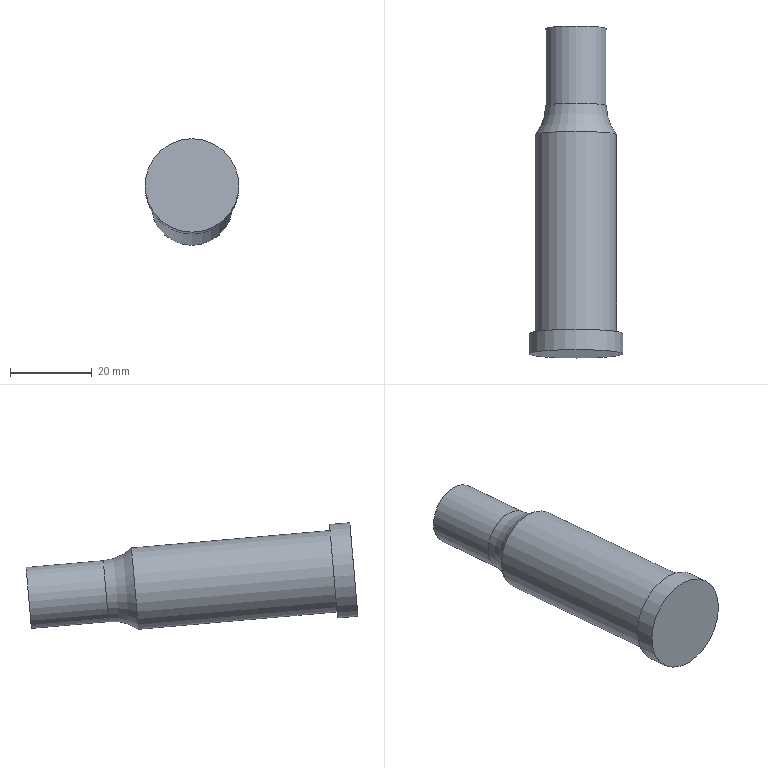Part | NX | features SPAS 20-80-18.00 2 | 1 solid | 7 faces | box 23 x 81.352 x 26.111 mm | volume 22338 mm3 | plane 3 | cylinder 3 | torus 1 | commonest cylinder face diameters 15 x1 20 x1 23 x1
STEP:
#1=CARTESIAN_POINT('',(-462.881,-59.853,-32.241));
#2=VERTEX_POINT('',#1);
#3=CARTESIAN_POINT('',(-462.881,-60.507,-39.712));
#4=DIRECTION('',(0.,0.9962,-0.08716));
#5=DIRECTION('',(0.,0.08716,0.9962));
#6=AXIS2_PLACEMENT_3D('',#3,#4,#5);
#7=CIRCLE('',#6,7.5);
#8=EDGE_CURVE('',#2,#2,#7,.F.);
#9=ORIENTED_EDGE('',*,*,#8,.F.);
#10=EDGE_LOOP('',(#9));
#11=FACE_BOUND('',#10,.T.);
#12=CARTESIAN_POINT('',(-462.881,-60.507,-39.712));
#13=DIRECTION('',(0.,0.9962,-0.08716));
#14=DIRECTION('',(0.,0.08716,0.9962));
#15=AXIS2_PLACEMENT_3D('',#12,#13,#14);
#16=PLANE('',#15);
#17=ADVANCED_FACE('',(#11),#16,.T.);
#18=CARTESIAN_POINT('',(-462.881,-80.088,-45.528));
#19=VERTEX_POINT('',#18);
#20=CARTESIAN_POINT('',(-462.881,-79.435,-38.056));
#21=DIRECTION('',(0.,-0.9962,0.08716));
#22=DIRECTION('',(0.,-0.08716,-0.9962));
#23=AXIS2_PLACEMENT_3D('',#20,#21,#22);
#24=CIRCLE('',#23,7.5);
#25=EDGE_CURVE('',#19,#19,#24,.F.);
#26=ORIENTED_EDGE('',*,*,#25,.T.);
#27=EDGE_LOOP('',(#26));
#28=FACE_BOUND('',#27,.T.);
#29=ORIENTED_EDGE('',*,*,#8,.T.);
#30=EDGE_LOOP('',(#29));
#31=FACE_BOUND('',#30,.T.);
#32=CARTESIAN_POINT('',(-462.881,-60.507,-39.712));
#33=DIRECTION('',(0.,-0.9962,0.08716));
#34=DIRECTION('',(0.,-0.08716,-0.9962));
#35=AXIS2_PLACEMENT_3D('',#32,#33,#34);
#36=CYLINDRICAL_SURFACE('',#35,7.5);
#37=ADVANCED_FACE('',(#28,#31),#36,.T.);
#38=CARTESIAN_POINT('',(-462.881,-134.35,-23.214));
#39=VERTEX_POINT('',#38);
#40=CARTESIAN_POINT('',(-462.881,-135.221,-33.175));
#41=DIRECTION('',(0.,0.9962,-0.08716));
#42=DIRECTION('',(0.,0.08716,0.9962));
#43=AXIS2_PLACEMENT_3D('',#40,#41,#42);
#44=CIRCLE('',#43,10.);
#45=EDGE_CURVE('',#39,#39,#44,.F.);
#46=ORIENTED_EDGE('',*,*,#45,.F.);
#47=EDGE_LOOP('',(#46));
#48=FACE_BOUND('',#47,.T.);
#49=CARTESIAN_POINT('',(-462.881,-85.695,-27.47));
#50=VERTEX_POINT('',#49);
#51=CARTESIAN_POINT('',(-462.881,-86.566,-37.432));
#52=DIRECTION('',(0.,0.9962,-0.08716));
#53=DIRECTION('',(0.,0.08716,0.9962));
#54=AXIS2_PLACEMENT_3D('',#51,#52,#53);
#55=CIRCLE('',#54,10.);
#56=EDGE_CURVE('',#50,#50,#55,.F.);
#57=ORIENTED_EDGE('',*,*,#56,.T.);
#58=EDGE_LOOP('',(#57));
#59=FACE_BOUND('',#58,.T.);
#60=CARTESIAN_POINT('',(-462.881,-83.777,-37.676));
#61=DIRECTION('',(0.,-0.9962,0.08716));
#62=DIRECTION('',(0.,-0.08716,-0.9962));
#63=AXIS2_PLACEMENT_3D('',#60,#61,#62);
#64=CYLINDRICAL_SURFACE('',#63,10.);
#65=ADVANCED_FACE('',(#48,#59),#64,.T.);
#66=CARTESIAN_POINT('',(-462.881,-139.2,-21.283));
#67=VERTEX_POINT('',#66);
#68=CARTESIAN_POINT('',(-462.881,-140.202,-32.74));
#69=DIRECTION('',(0.,0.9962,-0.08716));
#70=DIRECTION('',(0.,0.08716,0.9962));
#71=AXIS2_PLACEMENT_3D('',#68,#69,#70);
#72=CIRCLE('',#71,11.5);
#73=EDGE_CURVE('',#67,#67,#72,.T.);
#74=ORIENTED_EDGE('',*,*,#73,.F.);
#75=EDGE_LOOP('',(#74));
#76=FACE_BOUND('',#75,.T.);
#77=CARTESIAN_POINT('',(-462.881,-140.202,-32.74));
#78=DIRECTION('',(0.,-0.9962,0.08716));
#79=DIRECTION('',(0.,-0.08716,-0.9962));
#80=AXIS2_PLACEMENT_3D('',#77,#78,#79);
#81=PLANE('',#80);
#82=ADVANCED_FACE('',(#76),#81,.T.);
#83=ORIENTED_EDGE('',*,*,#45,.T.);
#84=EDGE_LOOP('',(#83));
#85=FACE_BOUND('',#84,.T.);
#86=CARTESIAN_POINT('',(-462.881,-136.224,-44.632));
#87=VERTEX_POINT('',#86);
#88=CARTESIAN_POINT('',(-462.881,-135.221,-33.175));
#89=DIRECTION('',(0.,-0.9962,0.08716));
#90=DIRECTION('',(0.,-0.08716,-0.9962));
#91=AXIS2_PLACEMENT_3D('',#88,#89,#90);
#92=CIRCLE('',#91,11.5);
#93=EDGE_CURVE('',#87,#87,#92,.T.);
#94=ORIENTED_EDGE('',*,*,#93,.F.);
#95=EDGE_LOOP('',(#94));
#96=FACE_BOUND('',#95,.T.);
#97=CARTESIAN_POINT('',(-462.881,-135.221,-33.175));
#98=DIRECTION('',(0.,0.9962,-0.08716));
#99=DIRECTION('',(0.,0.08716,0.9962));
#100=AXIS2_PLACEMENT_3D('',#97,#98,#99);
#101=PLANE('',#100);
#102=ADVANCED_FACE('',(#85,#96),#101,.T.);
#103=ORIENTED_EDGE('',*,*,#73,.T.);
#104=EDGE_LOOP('',(#103));
#105=FACE_BOUND('',#104,.T.);
#106=ORIENTED_EDGE('',*,*,#93,.T.);
#107=EDGE_LOOP('',(#106));
#108=FACE_BOUND('',#107,.T.);
#109=CARTESIAN_POINT('',(-462.881,-135.221,-33.175));
#110=DIRECTION('',(0.,-0.9962,0.08716));
#111=DIRECTION('',(0.,-0.08716,-0.9962));
#112=AXIS2_PLACEMENT_3D('',#109,#110,#111);
#113=CYLINDRICAL_SURFACE('',#112,11.5);
#114=ADVANCED_FACE('',(#105,#108),#113,.T.);
#115=ORIENTED_EDGE('',*,*,#25,.F.);
#116=EDGE_LOOP('',(#115));
#117=FACE_BOUND('',#116,.T.);
#118=ORIENTED_EDGE('',*,*,#56,.F.);
#119=EDGE_LOOP('',(#118));
#120=FACE_BOUND('',#119,.T.);
#121=CARTESIAN_POINT('',(-462.881,-79.435,-38.056));
#122=DIRECTION('',(0.,-0.9962,0.08716));
#123=DIRECTION('',(0.,-0.08716,-0.9962));
#124=AXIS2_PLACEMENT_3D('',#121,#122,#123);
#125=TOROIDAL_SURFACE('',#124,19.,11.5);
#126=ADVANCED_FACE('',(#117,#120),#125,.F.);
#127=CLOSED_SHELL('',(#17,#37,#65,#82,#102,#114,#126));
#128=MANIFOLD_SOLID_BREP('',#127);
#129=(LENGTH_UNIT()NAMED_UNIT(*)SI_UNIT(.MILLI.,.METRE.));
#130=UNCERTAINTY_MEASURE_WITH_UNIT(LENGTH_MEASURE(0.00001),#129,'','');
#131=(NAMED_UNIT(*)PLANE_ANGLE_UNIT()SI_UNIT($,.RADIAN.));
#132=(NAMED_UNIT(*)SI_UNIT($,.STERADIAN.)SOLID_ANGLE_UNIT());
#133=(GEOMETRIC_REPRESENTATION_CONTEXT(3)GLOBAL_UNCERTAINTY_ASSIGNED_CONTEXT((#130))GLOBAL_UNIT_ASSIGNED_CONTEXT((#129,#131,#132))REPRESENTATION_CONTEXT('',''));
#134=ADVANCED_BREP_SHAPE_REPRESENTATION('',(#128),#133);